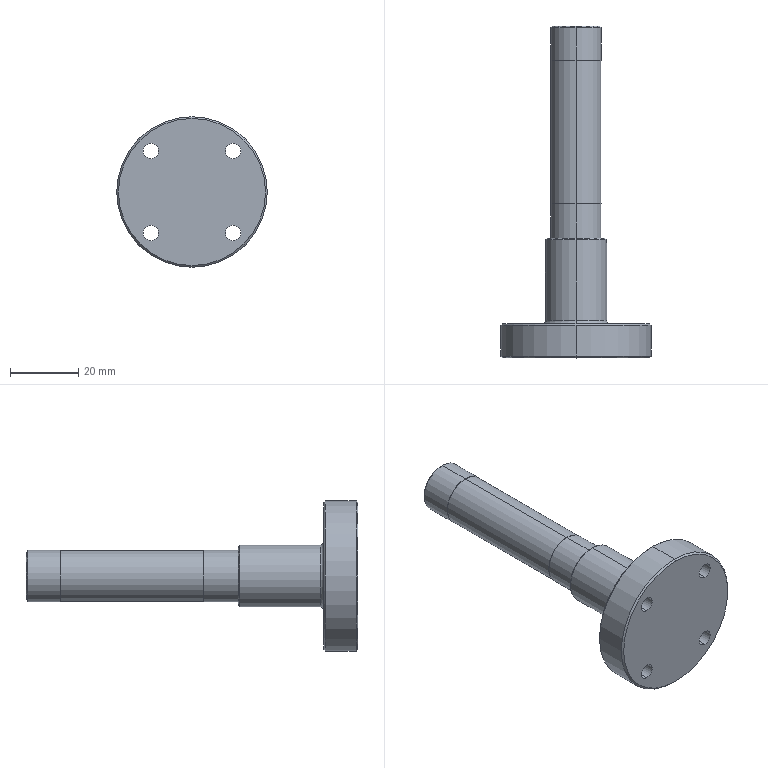Part | STEP file | ND25021-01-JDKM-03B-TL | 1 solid | 50 faces | box 44 x 97 x 44 mm | volume 30962 mm3 | cylinder 28 | cone 10 | plane 10 | torus 2 | commonest cylinder face diameters 4.5 x8 8 x8 15 x4 3.3 x2 14.8 x2 18 x2